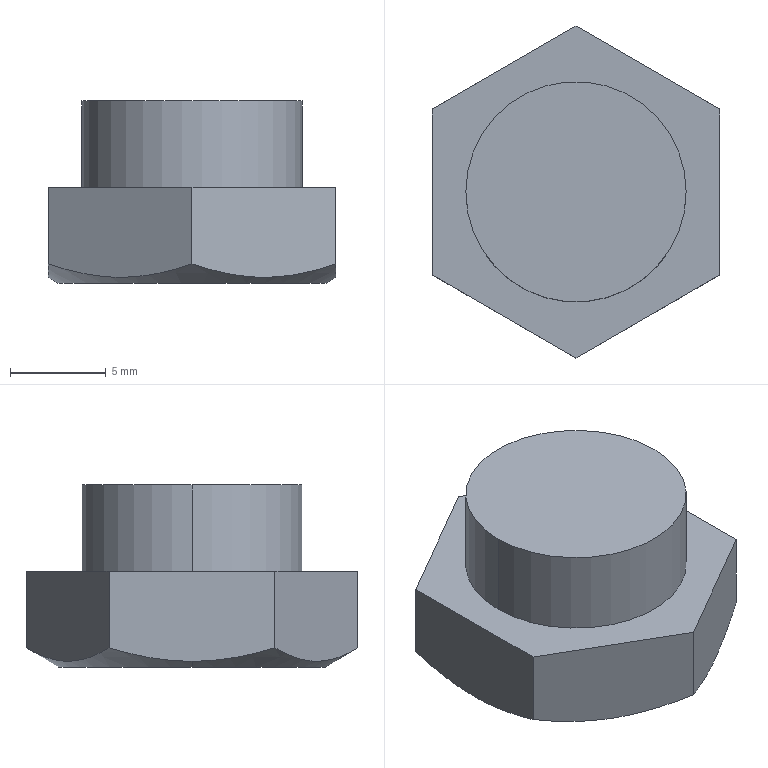Part | SolidWorks | features BaseBody 1 | 1 solid | 13 faces | box 15 x 17.321 x 9.5 mm | volume 1429 mm3 | plane 9 | cone 2 | cylinder 2 | commonest cylinder face diameters 11.5 x2
STEP:
#1=CARTESIAN_POINT('',(7.,0.,0.));
#2=VERTEX_POINT('',#1);
#3=CARTESIAN_POINT('',(-7.,0.,0.));
#4=VERTEX_POINT('',#3);
#5=CARTESIAN_POINT('',(0.,0.,0.));
#6=DIRECTION('',(0.,0.,1.));
#7=DIRECTION('',(1.,0.,0.));
#8=AXIS2_PLACEMENT_3D('',#5,#6,#7);
#9=CIRCLE('',#8,7.);
#10=EDGE_CURVE('',#2,#4,#9,.T.);
#11=ORIENTED_EDGE('',*,*,#10,.T.);
#12=CARTESIAN_POINT('',(-7.5,0.,0.3012));
#13=VERTEX_POINT('',#12);
#14=CARTESIAN_POINT('',(-8.67,0.,1.006));
#15=DIRECTION('',(-0.8566,0.,0.516));
#16=VECTOR('',#15,1000.);
#17=LINE('',#14,#16);
#18=EDGE_CURVE('',#4,#13,#17,.T.);
#19=ORIENTED_EDGE('',*,*,#18,.T.);
#20=CARTESIAN_POINT('',(-7.5,4.33,1.));
#21=VERTEX_POINT('',#20);
#22=CARTESIAN_POINT('',(-7.5,0.,0.3012));
#23=CARTESIAN_POINT('',(-7.5,0.3679,0.3012));
#24=CARTESIAN_POINT('',(-7.5,0.7378,0.3177));
#25=CARTESIAN_POINT('',(-7.5,1.469,0.3818));
#26=CARTESIAN_POINT('',(-7.5,1.832,0.4293));
#27=CARTESIAN_POINT('',(-7.5,2.913,0.612));
#28=CARTESIAN_POINT('',(-7.5,3.625,0.7876));
#29=CARTESIAN_POINT('',(-7.5,4.33,1.));
#30=B_SPLINE_CURVE_WITH_KNOTS('',3,(#22,#23,#24,#25,#26,#27,#28,#29),.UNSPECIFIED.,.F.,.F.,(4,2,2,4),(0.004386,0.005477,0.006569,0.008752),.UNSPECIFIED.);
#31=EDGE_CURVE('',#13,#21,#30,.T.);
#32=ORIENTED_EDGE('',*,*,#31,.T.);
#33=CARTESIAN_POINT('',(0.,8.66,1.));
#34=VERTEX_POINT('',#33);
#35=CARTESIAN_POINT('',(-7.5,4.33,1.));
#36=CARTESIAN_POINT('',(-6.889,4.683,0.7875));
#37=CARTESIAN_POINT('',(-6.273,5.039,0.6121));
#38=CARTESIAN_POINT('',(-5.027,5.758,0.3688));
#39=CARTESIAN_POINT('',(-4.397,6.122,0.3017));
#40=CARTESIAN_POINT('',(-3.439,6.675,0.3009));
#41=CARTESIAN_POINT('',(-3.118,6.86,0.3172));
#42=CARTESIAN_POINT('',(-2.483,7.226,0.3811));
#43=CARTESIAN_POINT('',(-2.169,7.408,0.4284));
#44=CARTESIAN_POINT('',(-1.23,7.95,0.6112));
#45=CARTESIAN_POINT('',(-0.6121,8.307,0.7871));
#46=CARTESIAN_POINT('',(0.,8.66,1.));
#47=B_SPLINE_CURVE_WITH_KNOTS('',3,(#35,#36,#37,#38,#39,#40,#41,#42,#43,#44,#45,#46),.UNSPECIFIED.,.F.,.F.,(4,2,2,2,2,4),(0.,0.002188,0.004376,0.00547,0.006564,0.008752),.UNSPECIFIED.);
#48=EDGE_CURVE('',#21,#34,#47,.T.);
#49=ORIENTED_EDGE('',*,*,#48,.T.);
#50=CARTESIAN_POINT('',(7.5,4.33,1.));
#51=VERTEX_POINT('',#50);
#52=CARTESIAN_POINT('',(0.,8.66,1.));
#53=CARTESIAN_POINT('',(0.6112,8.307,0.7875));
#54=CARTESIAN_POINT('',(1.227,7.952,0.6121));
#55=CARTESIAN_POINT('',(2.473,7.232,0.3688));
#56=CARTESIAN_POINT('',(3.103,6.869,0.3017));
#57=CARTESIAN_POINT('',(4.061,6.316,0.3009));
#58=CARTESIAN_POINT('',(4.382,6.13,0.3172));
#59=CARTESIAN_POINT('',(5.017,5.764,0.3811));
#60=CARTESIAN_POINT('',(5.331,5.582,0.4284));
#61=CARTESIAN_POINT('',(6.27,5.04,0.6112));
#62=CARTESIAN_POINT('',(6.888,4.684,0.7871));
#63=CARTESIAN_POINT('',(7.5,4.33,1.));
#64=B_SPLINE_CURVE_WITH_KNOTS('',3,(#52,#53,#54,#55,#56,#57,#58,#59,#60,#61,#62,#63),.UNSPECIFIED.,.F.,.F.,(4,2,2,2,2,4),(0.,0.002188,0.004376,0.00547,0.006564,0.008752),.UNSPECIFIED.);
#65=EDGE_CURVE('',#34,#51,#64,.T.);
#66=ORIENTED_EDGE('',*,*,#65,.T.);
#67=CARTESIAN_POINT('',(7.5,0.,0.3012));
#68=VERTEX_POINT('',#67);
#69=CARTESIAN_POINT('',(7.5,4.33,1.));
#70=CARTESIAN_POINT('',(7.5,3.623,0.787));
#71=CARTESIAN_POINT('',(7.5,2.91,0.6113));
#72=CARTESIAN_POINT('',(7.5,1.468,0.368));
#73=CARTESIAN_POINT('',(7.5,0.739,0.3012));
#74=CARTESIAN_POINT('',(7.5,0.,0.3012));
#75=B_SPLINE_CURVE_WITH_KNOTS('',3,(#69,#70,#71,#72,#73,#74),.UNSPECIFIED.,.F.,.F.,(4,2,4),(0.,0.002193,0.004386),.UNSPECIFIED.);
#76=EDGE_CURVE('',#51,#68,#75,.T.);
#77=ORIENTED_EDGE('',*,*,#76,.T.);
#78=CARTESIAN_POINT('',(8.67,0.,1.006));
#79=DIRECTION('',(0.8566,0.,0.516));
#80=VECTOR('',#79,1000.);
#81=LINE('',#78,#80);
#82=EDGE_CURVE('',#2,#68,#81,.T.);
#83=ORIENTED_EDGE('',*,*,#82,.F.);
#84=EDGE_LOOP('',(#11,#19,#32,#49,#66,#77,#83));
#85=FACE_OUTER_BOUND('',#84,.T.);
#86=CARTESIAN_POINT('',(0.,0.,1.006));
#87=DIRECTION('',(0.,0.,1.));
#88=DIRECTION('',(1.,0.,0.));
#89=AXIS2_PLACEMENT_3D('',#86,#87,#88);
#90=CONICAL_SURFACE('',#89,8.67,1.029);
#91=ADVANCED_FACE('',(#85),#90,.T.);
#92=CARTESIAN_POINT('',(-5.75,0.,9.5));
#93=VERTEX_POINT('',#92);
#94=CARTESIAN_POINT('',(5.75,0.,9.5));
#95=VERTEX_POINT('',#94);
#96=CARTESIAN_POINT('',(0.,0.,9.5));
#97=DIRECTION('',(0.,0.,-1.));
#98=DIRECTION('',(-1.,0.,0.));
#99=AXIS2_PLACEMENT_3D('',#96,#97,#98);
#100=CIRCLE('',#99,5.75);
#101=EDGE_CURVE('',#93,#95,#100,.T.);
#102=ORIENTED_EDGE('',*,*,#101,.T.);
#103=CARTESIAN_POINT('',(5.75,0.,5.));
#104=VERTEX_POINT('',#103);
#105=CARTESIAN_POINT('',(5.75,0.,9.5));
#106=DIRECTION('',(0.,0.,-1.));
#107=VECTOR('',#106,1000.);
#108=LINE('',#105,#107);
#109=EDGE_CURVE('',#95,#104,#108,.T.);
#110=ORIENTED_EDGE('',*,*,#109,.T.);
#111=CARTESIAN_POINT('',(-5.75,0.,5.));
#112=VERTEX_POINT('',#111);
#113=CARTESIAN_POINT('',(0.,0.,5.));
#114=DIRECTION('',(0.,0.,-1.));
#115=DIRECTION('',(-1.,0.,0.));
#116=AXIS2_PLACEMENT_3D('',#113,#114,#115);
#117=CIRCLE('',#116,5.75);
#118=EDGE_CURVE('',#112,#104,#117,.T.);
#119=ORIENTED_EDGE('',*,*,#118,.F.);
#120=CARTESIAN_POINT('',(-5.75,0.,9.5));
#121=DIRECTION('',(0.,0.,-1.));
#122=VECTOR('',#121,1000.);
#123=LINE('',#120,#122);
#124=EDGE_CURVE('',#93,#112,#123,.T.);
#125=ORIENTED_EDGE('',*,*,#124,.F.);
#126=EDGE_LOOP('',(#102,#110,#119,#125));
#127=FACE_OUTER_BOUND('',#126,.T.);
#128=CARTESIAN_POINT('',(0.,0.,9.5));
#129=DIRECTION('',(0.,0.,-1.));
#130=DIRECTION('',(-1.,0.,0.));
#131=AXIS2_PLACEMENT_3D('',#128,#129,#130);
#132=CYLINDRICAL_SURFACE('',#131,5.75);
#133=ADVANCED_FACE('',(#127),#132,.T.);
#134=ORIENTED_EDGE('',*,*,#10,.F.);
#135=CARTESIAN_POINT('',(0.,0.,0.));
#136=DIRECTION('',(0.,0.,1.));
#137=DIRECTION('',(1.,0.,0.));
#138=AXIS2_PLACEMENT_3D('',#135,#136,#137);
#139=CIRCLE('',#138,7.);
#140=EDGE_CURVE('',#4,#2,#139,.T.);
#141=ORIENTED_EDGE('',*,*,#140,.F.);
#142=EDGE_LOOP('',(#134,#141));
#143=FACE_OUTER_BOUND('',#142,.T.);
#144=CARTESIAN_POINT('',(0.,0.,0.));
#145=DIRECTION('',(0.,0.,1.));
#146=DIRECTION('',(1.,0.,0.));
#147=AXIS2_PLACEMENT_3D('',#144,#145,#146);
#148=PLANE('',#147);
#149=ADVANCED_FACE('',(#143),#148,.F.);
#150=ORIENTED_EDGE('',*,*,#18,.F.);
#151=ORIENTED_EDGE('',*,*,#140,.T.);
#152=ORIENTED_EDGE('',*,*,#82,.T.);
#153=CARTESIAN_POINT('',(7.5,-4.33,1.));
#154=VERTEX_POINT('',#153);
#155=CARTESIAN_POINT('',(7.5,0.,0.3012));
#156=CARTESIAN_POINT('',(7.5,-0.3679,0.3012));
#157=CARTESIAN_POINT('',(7.5,-0.7378,0.3177));
#158=CARTESIAN_POINT('',(7.5,-1.469,0.3818));
#159=CARTESIAN_POINT('',(7.5,-1.832,0.4293));
#160=CARTESIAN_POINT('',(7.5,-2.913,0.612));
#161=CARTESIAN_POINT('',(7.5,-3.625,0.7876));
#162=CARTESIAN_POINT('',(7.5,-4.33,1.));
#163=B_SPLINE_CURVE_WITH_KNOTS('',3,(#155,#156,#157,#158,#159,#160,#161,#162),.UNSPECIFIED.,.F.,.F.,(4,2,2,4),(0.004386,0.005477,0.006569,0.008752),.UNSPECIFIED.);
#164=EDGE_CURVE('',#68,#154,#163,.T.);
#165=ORIENTED_EDGE('',*,*,#164,.T.);
#166=CARTESIAN_POINT('',(0.,-8.66,1.));
#167=VERTEX_POINT('',#166);
#168=CARTESIAN_POINT('',(7.5,-4.33,1.));
#169=CARTESIAN_POINT('',(6.889,-4.683,0.7875));
#170=CARTESIAN_POINT('',(6.273,-5.039,0.6121));
#171=CARTESIAN_POINT('',(5.027,-5.758,0.3688));
#172=CARTESIAN_POINT('',(4.397,-6.122,0.3017));
#173=CARTESIAN_POINT('',(3.439,-6.675,0.3009));
#174=CARTESIAN_POINT('',(3.118,-6.86,0.3172));
#175=CARTESIAN_POINT('',(2.483,-7.226,0.3811));
#176=CARTESIAN_POINT('',(2.169,-7.408,0.4284));
#177=CARTESIAN_POINT('',(1.23,-7.95,0.6112));
#178=CARTESIAN_POINT('',(0.6121,-8.307,0.7871));
#179=CARTESIAN_POINT('',(0.,-8.66,1.));
#180=B_SPLINE_CURVE_WITH_KNOTS('',3,(#168,#169,#170,#171,#172,#173,#174,#175,#176,#177,#178,#179),.UNSPECIFIED.,.F.,.F.,(4,2,2,2,2,4),(0.,0.002188,0.004376,0.00547,0.006564,0.008752),.UNSPECIFIED.);
#181=EDGE_CURVE('',#154,#167,#180,.T.);
#182=ORIENTED_EDGE('',*,*,#181,.T.);
#183=CARTESIAN_POINT('',(-7.5,-4.33,1.));
#184=VERTEX_POINT('',#183);
#185=CARTESIAN_POINT('',(0.,-8.66,1.));
#186=CARTESIAN_POINT('',(-0.6112,-8.307,0.7875));
#187=CARTESIAN_POINT('',(-1.227,-7.952,0.6121));
#188=CARTESIAN_POINT('',(-2.473,-7.232,0.3688));
#189=CARTESIAN_POINT('',(-3.103,-6.869,0.3017));
#190=CARTESIAN_POINT('',(-4.061,-6.316,0.3009));
#191=CARTESIAN_POINT('',(-4.382,-6.13,0.3172));
#192=CARTESIAN_POINT('',(-5.017,-5.764,0.3811));
#193=CARTESIAN_POINT('',(-5.331,-5.582,0.4284));
#194=CARTESIAN_POINT('',(-6.27,-5.04,0.6112));
#195=CARTESIAN_POINT('',(-6.888,-4.684,0.7871));
#196=CARTESIAN_POINT('',(-7.5,-4.33,1.));
#197=B_SPLINE_CURVE_WITH_KNOTS('',3,(#185,#186,#187,#188,#189,#190,#191,#192,#193,#194,#195,#196),.UNSPECIFIED.,.F.,.F.,(4,2,2,2,2,4),(0.,0.002188,0.004376,0.00547,0.006564,0.008752),.UNSPECIFIED.);
#198=EDGE_CURVE('',#167,#184,#197,.T.);
#199=ORIENTED_EDGE('',*,*,#198,.T.);
#200=CARTESIAN_POINT('',(-7.5,-4.33,1.));
#201=CARTESIAN_POINT('',(-7.5,-3.623,0.787));
#202=CARTESIAN_POINT('',(-7.5,-2.91,0.6113));
#203=CARTESIAN_POINT('',(-7.5,-1.468,0.368));
#204=CARTESIAN_POINT('',(-7.5,-0.739,0.3012));
#205=CARTESIAN_POINT('',(-7.5,0.,0.3012));
#206=B_SPLINE_CURVE_WITH_KNOTS('',3,(#200,#201,#202,#203,#204,#205),.UNSPECIFIED.,.F.,.F.,(4,2,4),(0.,0.002193,0.004386),.UNSPECIFIED.);
#207=EDGE_CURVE('',#184,#13,#206,.T.);
#208=ORIENTED_EDGE('',*,*,#207,.T.);
#209=EDGE_LOOP('',(#150,#151,#152,#165,#182,#199,#208));
#210=FACE_OUTER_BOUND('',#209,.T.);
#211=CARTESIAN_POINT('',(0.,0.,1.006));
#212=DIRECTION('',(0.,0.,1.));
#213=DIRECTION('',(1.,0.,0.));
#214=AXIS2_PLACEMENT_3D('',#211,#212,#213);
#215=CONICAL_SURFACE('',#214,8.67,1.029);
#216=ADVANCED_FACE('',(#210),#215,.T.);
#217=CARTESIAN_POINT('',(7.5,-4.33,5.));
#218=VERTEX_POINT('',#217);
#219=CARTESIAN_POINT('',(7.5,-4.33,5.));
#220=DIRECTION('',(0.,0.,-1.));
#221=VECTOR('',#220,1000.);
#222=LINE('',#219,#221);
#223=EDGE_CURVE('',#218,#154,#222,.T.);
#224=ORIENTED_EDGE('',*,*,#223,.F.);
#225=CARTESIAN_POINT('',(0.,-8.66,5.));
#226=VERTEX_POINT('',#225);
#227=CARTESIAN_POINT('',(0.,-8.66,5.));
#228=DIRECTION('',(0.866,0.5,0.));
#229=VECTOR('',#228,1000.);
#230=LINE('',#227,#229);
#231=EDGE_CURVE('',#226,#218,#230,.T.);
#232=ORIENTED_EDGE('',*,*,#231,.F.);
#233=CARTESIAN_POINT('',(0.,-8.66,5.));
#234=DIRECTION('',(0.,0.,1.));
#235=VECTOR('',#234,1000.);
#236=LINE('',#233,#235);
#237=EDGE_CURVE('',#167,#226,#236,.T.);
#238=ORIENTED_EDGE('',*,*,#237,.F.);
#239=ORIENTED_EDGE('',*,*,#181,.F.);
#240=EDGE_LOOP('',(#224,#232,#238,#239));
#241=FACE_OUTER_BOUND('',#240,.T.);
#242=CARTESIAN_POINT('',(0.,-8.66,5.));
#243=DIRECTION('',(-0.5,0.866,0.));
#244=DIRECTION('',(-0.866,-0.5,0.));
#245=AXIS2_PLACEMENT_3D('',#242,#243,#244);
#246=PLANE('',#245);
#247=ADVANCED_FACE('',(#241),#246,.F.);
#248=CARTESIAN_POINT('',(7.5,4.33,5.));
#249=VERTEX_POINT('',#248);
#250=CARTESIAN_POINT('',(7.5,4.33,5.));
#251=DIRECTION('',(0.,0.,-1.));
#252=VECTOR('',#251,1000.);
#253=LINE('',#250,#252);
#254=EDGE_CURVE('',#249,#51,#253,.T.);
#255=ORIENTED_EDGE('',*,*,#254,.F.);
#256=CARTESIAN_POINT('',(7.5,-4.33,5.));
#257=DIRECTION('',(0.,1.,0.));
#258=VECTOR('',#257,1000.);
#259=LINE('',#256,#258);
#260=EDGE_CURVE('',#218,#249,#259,.T.);
#261=ORIENTED_EDGE('',*,*,#260,.F.);
#262=ORIENTED_EDGE('',*,*,#223,.T.);
#263=ORIENTED_EDGE('',*,*,#164,.F.);
#264=ORIENTED_EDGE('',*,*,#76,.F.);
#265=EDGE_LOOP('',(#255,#261,#262,#263,#264));
#266=FACE_OUTER_BOUND('',#265,.T.);
#267=CARTESIAN_POINT('',(7.5,-4.33,5.));
#268=DIRECTION('',(-1.,0.,0.));
#269=DIRECTION('',(0.,-1.,0.));
#270=AXIS2_PLACEMENT_3D('',#267,#268,#269);
#271=PLANE('',#270);
#272=ADVANCED_FACE('',(#266),#271,.F.);
#273=CARTESIAN_POINT('',(0.,8.66,5.));
#274=VERTEX_POINT('',#273);
#275=CARTESIAN_POINT('',(0.,8.66,5.));
#276=DIRECTION('',(0.,0.,-1.));
#277=VECTOR('',#276,1000.);
#278=LINE('',#275,#277);
#279=EDGE_CURVE('',#274,#34,#278,.T.);
#280=ORIENTED_EDGE('',*,*,#279,.F.);
#281=CARTESIAN_POINT('',(7.5,4.33,5.));
#282=DIRECTION('',(-0.866,0.5,0.));
#283=VECTOR('',#282,1000.);
#284=LINE('',#281,#283);
#285=EDGE_CURVE('',#249,#274,#284,.T.);
#286=ORIENTED_EDGE('',*,*,#285,.F.);
#287=ORIENTED_EDGE('',*,*,#254,.T.);
#288=ORIENTED_EDGE('',*,*,#65,.F.);
#289=EDGE_LOOP('',(#280,#286,#287,#288));
#290=FACE_OUTER_BOUND('',#289,.T.);
#291=CARTESIAN_POINT('',(7.5,4.33,5.));
#292=DIRECTION('',(-0.5,-0.866,0.));
#293=DIRECTION('',(0.866,-0.5,0.));
#294=AXIS2_PLACEMENT_3D('',#291,#292,#293);
#295=PLANE('',#294);
#296=ADVANCED_FACE('',(#290),#295,.F.);
#297=CARTESIAN_POINT('',(-7.5,4.33,5.));
#298=VERTEX_POINT('',#297);
#299=CARTESIAN_POINT('',(-7.5,4.33,5.));
#300=DIRECTION('',(0.,0.,-1.));
#301=VECTOR('',#300,1000.);
#302=LINE('',#299,#301);
#303=EDGE_CURVE('',#298,#21,#302,.T.);
#304=ORIENTED_EDGE('',*,*,#303,.F.);
#305=CARTESIAN_POINT('',(0.,8.66,5.));
#306=DIRECTION('',(-0.866,-0.5,0.));
#307=VECTOR('',#306,1000.);
#308=LINE('',#305,#307);
#309=EDGE_CURVE('',#274,#298,#308,.T.);
#310=ORIENTED_EDGE('',*,*,#309,.F.);
#311=ORIENTED_EDGE('',*,*,#279,.T.);
#312=ORIENTED_EDGE('',*,*,#48,.F.);
#313=EDGE_LOOP('',(#304,#310,#311,#312));
#314=FACE_OUTER_BOUND('',#313,.T.);
#315=CARTESIAN_POINT('',(0.,8.66,5.));
#316=DIRECTION('',(0.5,-0.866,0.));
#317=DIRECTION('',(0.866,0.5,0.));
#318=AXIS2_PLACEMENT_3D('',#315,#316,#317);
#319=PLANE('',#318);
#320=ADVANCED_FACE('',(#314),#319,.F.);
#321=CARTESIAN_POINT('',(-7.5,-4.33,5.));
#322=VERTEX_POINT('',#321);
#323=CARTESIAN_POINT('',(-7.5,-4.33,5.));
#324=DIRECTION('',(0.,0.,-1.));
#325=VECTOR('',#324,1000.);
#326=LINE('',#323,#325);
#327=EDGE_CURVE('',#322,#184,#326,.T.);
#328=ORIENTED_EDGE('',*,*,#327,.F.);
#329=CARTESIAN_POINT('',(-7.5,4.33,5.));
#330=DIRECTION('',(0.,-1.,0.));
#331=VECTOR('',#330,1000.);
#332=LINE('',#329,#331);
#333=EDGE_CURVE('',#298,#322,#332,.T.);
#334=ORIENTED_EDGE('',*,*,#333,.F.);
#335=ORIENTED_EDGE('',*,*,#303,.T.);
#336=ORIENTED_EDGE('',*,*,#31,.F.);
#337=ORIENTED_EDGE('',*,*,#207,.F.);
#338=EDGE_LOOP('',(#328,#334,#335,#336,#337));
#339=FACE_OUTER_BOUND('',#338,.T.);
#340=CARTESIAN_POINT('',(-7.5,4.33,5.));
#341=DIRECTION('',(1.,0.,0.));
#342=DIRECTION('',(0.,0.,-1.));
#343=AXIS2_PLACEMENT_3D('',#340,#341,#342);
#344=PLANE('',#343);
#345=ADVANCED_FACE('',(#339),#344,.F.);
#346=ORIENTED_EDGE('',*,*,#237,.T.);
#347=CARTESIAN_POINT('',(-7.5,-4.33,5.));
#348=DIRECTION('',(0.866,-0.5,0.));
#349=VECTOR('',#348,1000.);
#350=LINE('',#347,#349);
#351=EDGE_CURVE('',#322,#226,#350,.T.);
#352=ORIENTED_EDGE('',*,*,#351,.F.);
#353=ORIENTED_EDGE('',*,*,#327,.T.);
#354=ORIENTED_EDGE('',*,*,#198,.F.);
#355=EDGE_LOOP('',(#346,#352,#353,#354));
#356=FACE_OUTER_BOUND('',#355,.T.);
#357=CARTESIAN_POINT('',(-7.5,-4.33,5.));
#358=DIRECTION('',(0.5,0.866,0.));
#359=DIRECTION('',(-0.866,0.5,0.));
#360=AXIS2_PLACEMENT_3D('',#357,#358,#359);
#361=PLANE('',#360);
#362=ADVANCED_FACE('',(#356),#361,.F.);
#363=ORIENTED_EDGE('',*,*,#231,.T.);
#364=ORIENTED_EDGE('',*,*,#260,.T.);
#365=ORIENTED_EDGE('',*,*,#285,.T.);
#366=ORIENTED_EDGE('',*,*,#309,.T.);
#367=ORIENTED_EDGE('',*,*,#333,.T.);
#368=ORIENTED_EDGE('',*,*,#351,.T.);
#369=EDGE_LOOP('',(#363,#364,#365,#366,#367,#368));
#370=FACE_OUTER_BOUND('',#369,.T.);
#371=ORIENTED_EDGE('',*,*,#118,.T.);
#372=CARTESIAN_POINT('',(0.,0.,5.));
#373=DIRECTION('',(0.,0.,-1.));
#374=DIRECTION('',(-1.,0.,0.));
#375=AXIS2_PLACEMENT_3D('',#372,#373,#374);
#376=CIRCLE('',#375,5.75);
#377=EDGE_CURVE('',#104,#112,#376,.T.);
#378=ORIENTED_EDGE('',*,*,#377,.T.);
#379=EDGE_LOOP('',(#371,#378));
#380=FACE_BOUND('',#379,.T.);
#381=CARTESIAN_POINT('',(0.,0.,5.));
#382=DIRECTION('',(0.,0.,1.));
#383=DIRECTION('',(1.,0.,0.));
#384=AXIS2_PLACEMENT_3D('',#381,#382,#383);
#385=PLANE('',#384);
#386=ADVANCED_FACE('',(#370,#380),#385,.T.);
#387=ORIENTED_EDGE('',*,*,#109,.F.);
#388=CARTESIAN_POINT('',(0.,0.,9.5));
#389=DIRECTION('',(0.,0.,-1.));
#390=DIRECTION('',(-1.,0.,0.));
#391=AXIS2_PLACEMENT_3D('',#388,#389,#390);
#392=CIRCLE('',#391,5.75);
#393=EDGE_CURVE('',#95,#93,#392,.T.);
#394=ORIENTED_EDGE('',*,*,#393,.T.);
#395=ORIENTED_EDGE('',*,*,#124,.T.);
#396=ORIENTED_EDGE('',*,*,#377,.F.);
#397=EDGE_LOOP('',(#387,#394,#395,#396));
#398=FACE_OUTER_BOUND('',#397,.T.);
#399=CARTESIAN_POINT('',(0.,0.,9.5));
#400=DIRECTION('',(0.,0.,-1.));
#401=DIRECTION('',(-1.,0.,0.));
#402=AXIS2_PLACEMENT_3D('',#399,#400,#401);
#403=CYLINDRICAL_SURFACE('',#402,5.75);
#404=ADVANCED_FACE('',(#398),#403,.T.);
#405=ORIENTED_EDGE('',*,*,#101,.F.);
#406=ORIENTED_EDGE('',*,*,#393,.F.);
#407=EDGE_LOOP('',(#405,#406));
#408=FACE_OUTER_BOUND('',#407,.T.);
#409=CARTESIAN_POINT('',(0.,0.,9.5));
#410=DIRECTION('',(0.,0.,1.));
#411=DIRECTION('',(1.,0.,0.));
#412=AXIS2_PLACEMENT_3D('',#409,#410,#411);
#413=PLANE('',#412);
#414=ADVANCED_FACE('',(#408),#413,.T.);
#415=CLOSED_SHELL('',(#91,#133,#149,#216,#247,#272,#296,#320,#345,#362,#386,#404,#414));
#416=MANIFOLD_SOLID_BREP('',#415);
#417=CARTESIAN_POINT('',(0.,0.,0.));
#418=DIRECTION('',(0.,0.,1.));
#419=DIRECTION('',(1.,0.,0.));
#420=AXIS2_PLACEMENT_3D('',#417,#418,#419);
#421=(LENGTH_UNIT()NAMED_UNIT(*)SI_UNIT(.MILLI.,.METRE.));
#422=UNCERTAINTY_MEASURE_WITH_UNIT(LENGTH_MEASURE(0.00001),#421,'','');
#423=(NAMED_UNIT(*)PLANE_ANGLE_UNIT()SI_UNIT($,.RADIAN.));
#424=(NAMED_UNIT(*)SI_UNIT($,.STERADIAN.)SOLID_ANGLE_UNIT());
#425=(GEOMETRIC_REPRESENTATION_CONTEXT(3)GLOBAL_UNCERTAINTY_ASSIGNED_CONTEXT((#422))GLOBAL_UNIT_ASSIGNED_CONTEXT((#421,#423,#424))REPRESENTATION_CONTEXT('',''));
#426=ADVANCED_BREP_SHAPE_REPRESENTATION('',(#416,#420),#425);